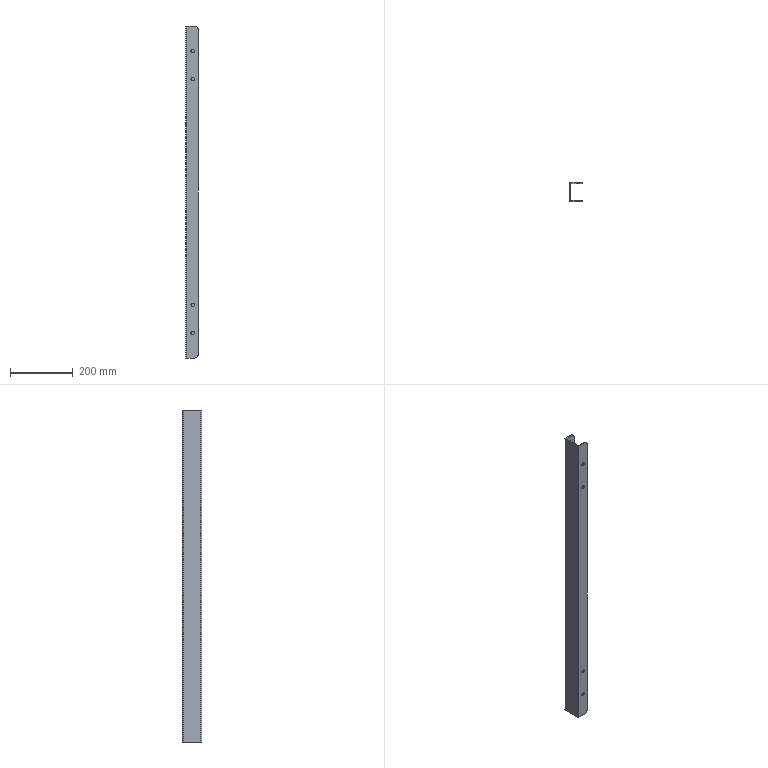Part | SolidWorks | features ICE 2, Cut 1, Fillet 1, FlatPattern 1, SMBaseFlange 1, SheetMetal 1 | 1 solid | 63 faces | box 40 x 62 x 1060 mm | volume 421378 mm3 | cylinder 35 | plane 28 | commonest cylinder face diameters 10 x15 11 x8 12.8 x4 24 x4 0.4 x2 6.4 x2